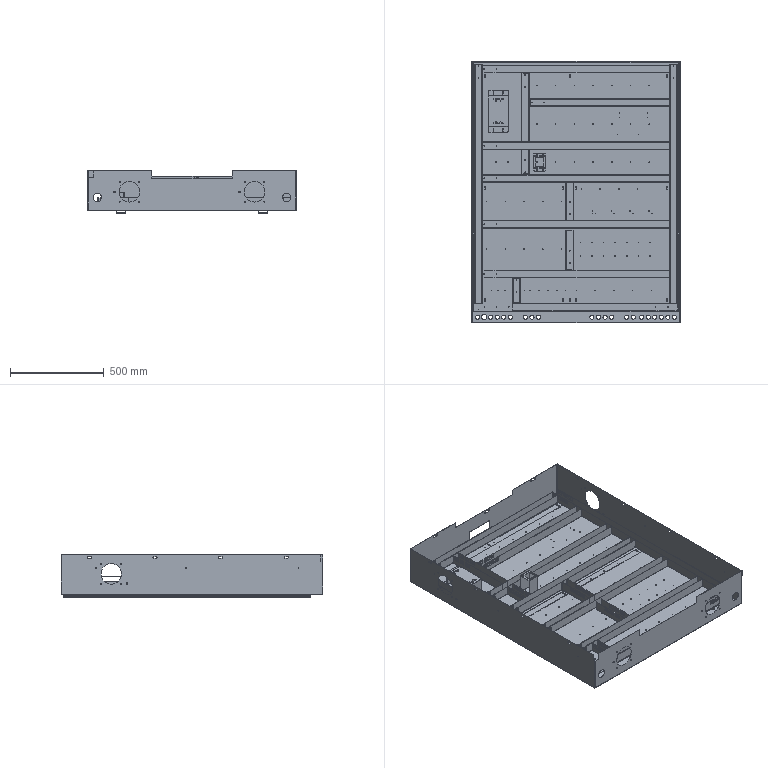Part | SolidWorks | features InContextFeatHolder 4, LayoutProfileFeature 1 | 23 solids | 2684 faces | box 1110 x 1395 x 228 mm | volume 9072587 mm3 | plane 1636 | cylinder 1038 | spline 10 | commonest cylinder face diameters 3.3 x514 6 x70 5 x68 3 x56 0.4 x42 22 x40